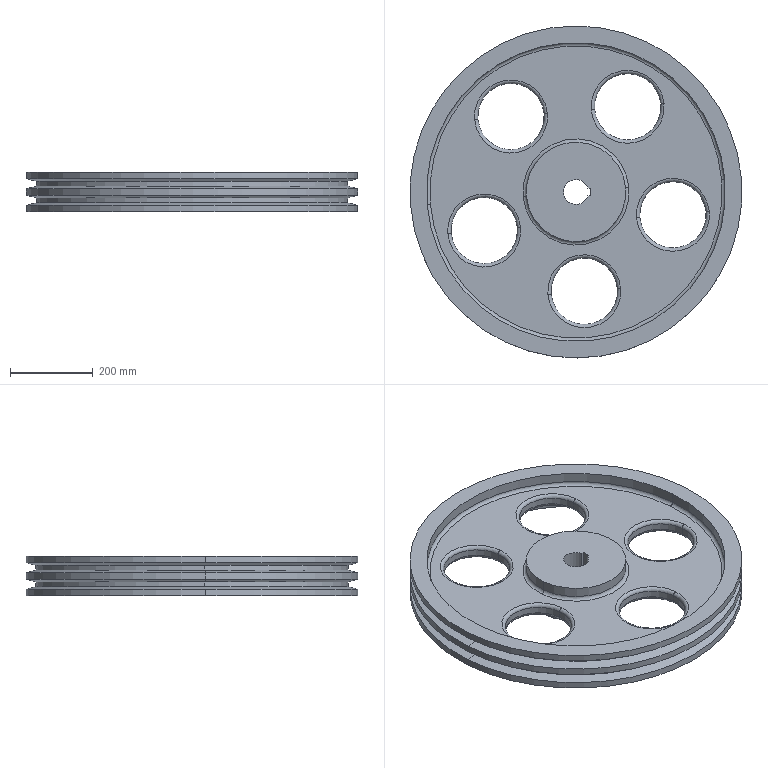Part | SolidWorks | features BaseBody 1 | 1 solid | 75 faces | box 800 x 800 x 96 mm | volume 19493406 mm3 | cylinder 30 | torus 28 | plane 9 | cone 8 | commonest cylinder face diameters 160 x10 800 x6 240 x4 720 x4 752 x4 60 x2